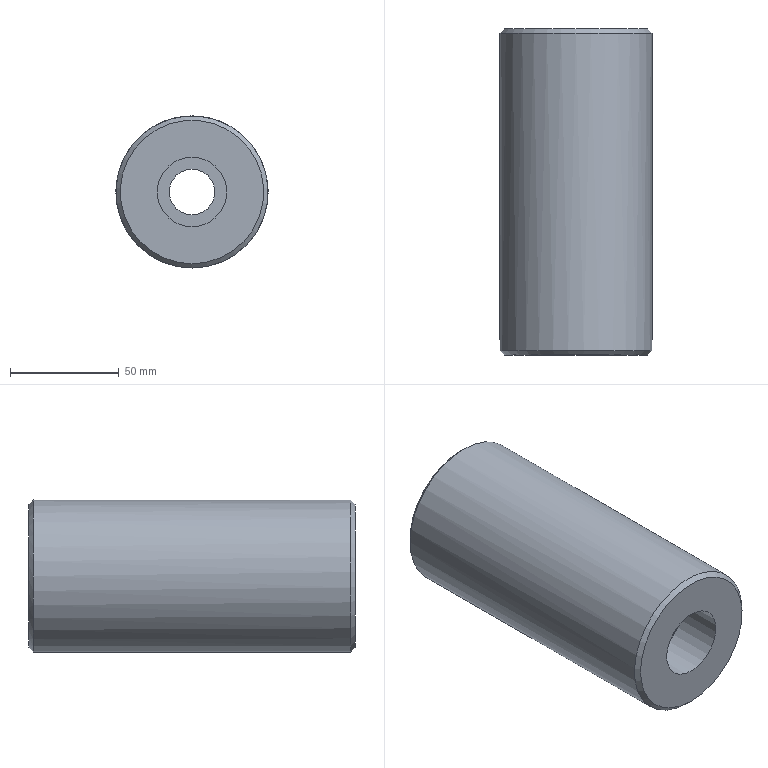Part | STEP file | solid 107 | 1 solid | 8 faces | box 70 x 150 x 70 mm | volume 514377 mm3 | plane 3 | cylinder 3 | cone 2 | commonest cylinder face diameters 21 x1 32 x1 70 x1